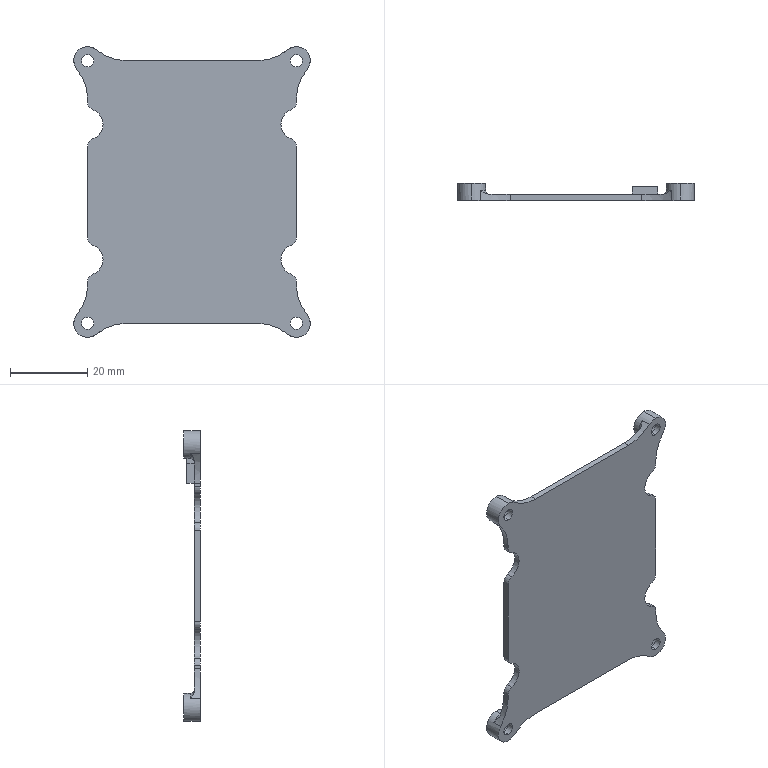Part | SolidWorks | features Fillet 3, ICE 2, Extrusion 1 | 1 solid | 75 faces | box 61.2 x 4.4 x 75.2 mm | volume 6161 mm3 | cylinder 44 | plane 25 | torus 6 | commonest cylinder face diameters 3.2 x8 4 x8 5.3 x8 7.2 x8 24 x8 8 x4